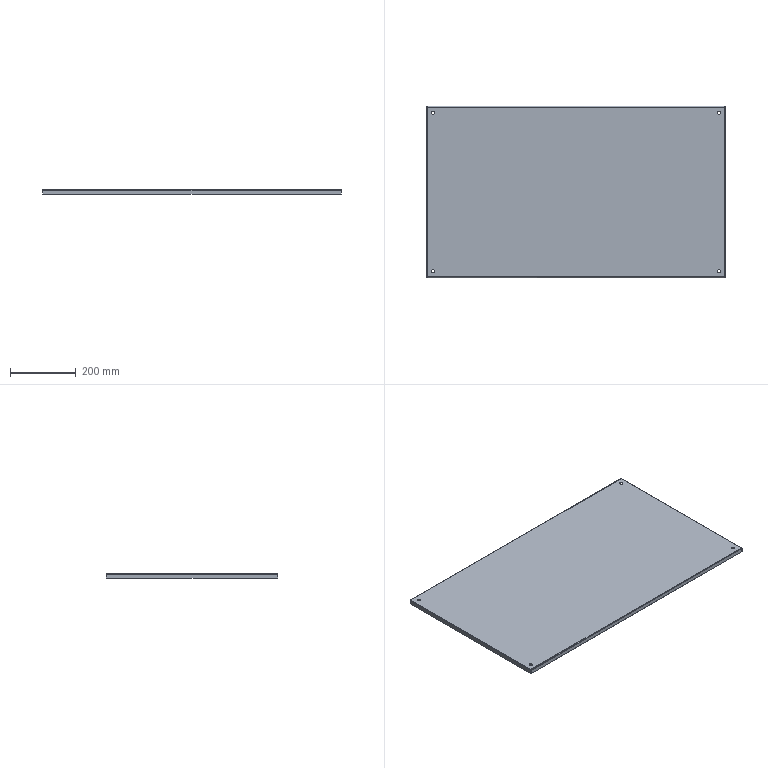Part | SolidWorks | features 3DProfileFeature 1, EdgeFlange 1, FlatPattern 1, HoleWzd 1, SMBaseFlange 1, SheetMetal 1 | 1 solid | 46 faces | box 907 x 520 x 13.8 mm | volume 606294 mm3 | plane 22 | cylinder 16 | spline 8 | commonest cylinder face diameters 9 x8 2 x4 4.4 x4